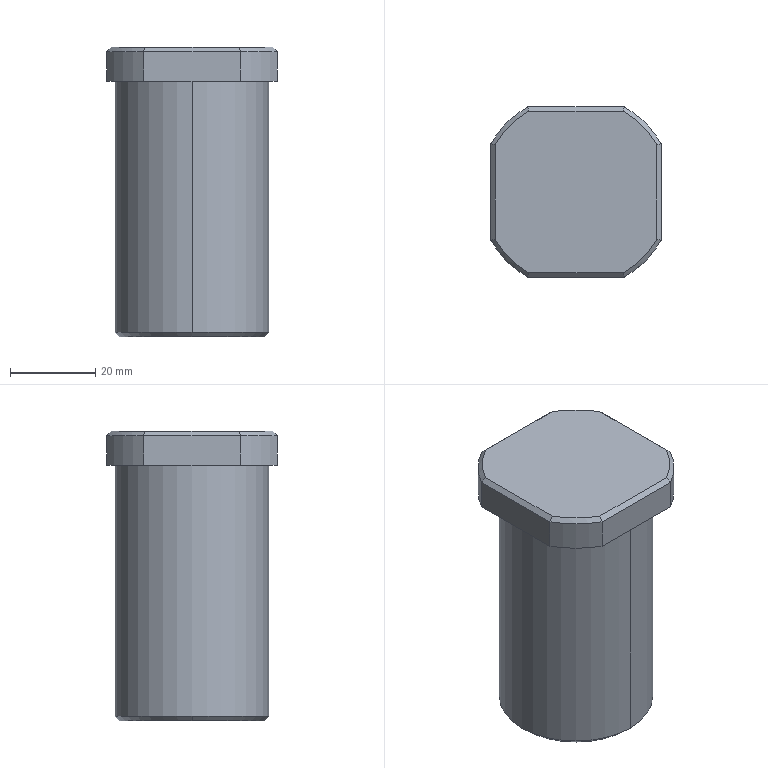Part | Creo | 1 solid | 30 faces | box 40 x 40 x 68 mm | volume 63302 mm3 | plane 12 | cylinder 10 | cone 8 | commonest cylinder face diameters 46 x4 14 x2 16 x2 36 x2
STEP:
#1=CARTESIAN_POINT('',(50.,216.995,-364.));
#2=VERTEX_POINT('',#1);
#3=CARTESIAN_POINT('',(67.,199.995,-364.));
#4=VERTEX_POINT('',#3);
#5=CARTESIAN_POINT('',(50.,199.995,-364.));
#6=DIRECTION('',(0.,0.,-1.));
#7=DIRECTION('',(0.,1.,0.));
#8=AXIS2_PLACEMENT_3D('',#5,#6,#7);
#9=CIRCLE('',#8,17.);
#10=EDGE_CURVE('',#2,#4,#9,.T.);
#11=ORIENTED_EDGE('',*,*,#10,.F.);
#12=CARTESIAN_POINT('',(33.,199.995,-364.));
#13=VERTEX_POINT('',#12);
#14=CARTESIAN_POINT('',(50.,199.995,-364.));
#15=DIRECTION('',(0.,0.,-1.));
#16=DIRECTION('',(-1.,0.,0.));
#17=AXIS2_PLACEMENT_3D('',#14,#15,#16);
#18=CIRCLE('',#17,17.);
#19=EDGE_CURVE('',#13,#2,#18,.T.);
#20=ORIENTED_EDGE('',*,*,#19,.F.);
#21=CARTESIAN_POINT('',(50.,199.995,-364.));
#22=DIRECTION('',(0.,0.,-1.));
#23=DIRECTION('',(1.,0.,0.));
#24=AXIS2_PLACEMENT_3D('',#21,#22,#23);
#25=CIRCLE('',#24,17.);
#26=EDGE_CURVE('',#4,#13,#25,.T.);
#27=ORIENTED_EDGE('',*,*,#26,.F.);
#28=EDGE_LOOP('',(#11,#20,#27));
#29=FACE_OUTER_BOUND('',#28,.F.);
#30=CARTESIAN_POINT('',(42.,199.995,-364.));
#31=VERTEX_POINT('',#30);
#32=CARTESIAN_POINT('',(58.,199.995,-364.));
#33=VERTEX_POINT('',#32);
#34=CARTESIAN_POINT('',(50.,199.995,-364.));
#35=DIRECTION('',(0.,0.,1.));
#36=DIRECTION('',(-1.,0.,0.));
#37=AXIS2_PLACEMENT_3D('',#34,#35,#36);
#38=CIRCLE('',#37,8.);
#39=EDGE_CURVE('',#31,#33,#38,.T.);
#40=ORIENTED_EDGE('',*,*,#39,.F.);
#41=CARTESIAN_POINT('',(50.,199.995,-364.));
#42=DIRECTION('',(0.,0.,1.));
#43=DIRECTION('',(1.,0.,0.));
#44=AXIS2_PLACEMENT_3D('',#41,#42,#43);
#45=CIRCLE('',#44,8.);
#46=EDGE_CURVE('',#33,#31,#45,.T.);
#47=ORIENTED_EDGE('',*,*,#46,.F.);
#48=EDGE_LOOP('',(#40,#47));
#49=FACE_BOUND('',#48,.F.);
#50=CARTESIAN_POINT('',(50.,199.995,-364.));
#51=DIRECTION('',(0.,0.,-1.));
#52=DIRECTION('',(0.,1.,0.));
#53=AXIS2_PLACEMENT_3D('',#50,#51,#52);
#54=PLANE('',#53);
#55=ADVANCED_FACE('',(#29,#49),#54,.T.);
#56=CARTESIAN_POINT('',(50.,217.995,-363.));
#57=VERTEX_POINT('',#56);
#58=CARTESIAN_POINT('',(68.,199.995,-363.));
#59=VERTEX_POINT('',#58);
#60=CARTESIAN_POINT('',(50.,199.995,-363.));
#61=DIRECTION('',(0.,0.,-1.));
#62=DIRECTION('',(0.,1.,0.));
#63=AXIS2_PLACEMENT_3D('',#60,#61,#62);
#64=CIRCLE('',#63,18.);
#65=EDGE_CURVE('',#57,#59,#64,.T.);
#66=ORIENTED_EDGE('',*,*,#65,.F.);
#67=CARTESIAN_POINT('',(32.,199.995,-363.));
#68=VERTEX_POINT('',#67);
#69=CARTESIAN_POINT('',(50.,199.995,-363.));
#70=DIRECTION('',(0.,0.,-1.));
#71=DIRECTION('',(-1.,0.,0.));
#72=AXIS2_PLACEMENT_3D('',#69,#70,#71);
#73=CIRCLE('',#72,18.);
#74=EDGE_CURVE('',#68,#57,#73,.T.);
#75=ORIENTED_EDGE('',*,*,#74,.F.);
#76=CARTESIAN_POINT('',(33.,199.995,-364.));
#77=DIRECTION('',(-0.7071,0.,0.7071));
#78=VECTOR('',#77,1.414);
#79=LINE('',#76,#78);
#80=EDGE_CURVE('',#13,#68,#79,.T.);
#81=ORIENTED_EDGE('',*,*,#80,.F.);
#82=ORIENTED_EDGE('',*,*,#19,.T.);
#83=ORIENTED_EDGE('',*,*,#10,.T.);
#84=CARTESIAN_POINT('',(67.,199.995,-364.));
#85=DIRECTION('',(0.7071,0.,0.7071));
#86=VECTOR('',#85,1.414);
#87=LINE('',#84,#86);
#88=EDGE_CURVE('',#4,#59,#87,.T.);
#89=ORIENTED_EDGE('',*,*,#88,.T.);
#90=EDGE_LOOP('',(#66,#75,#81,#82,#83,#89));
#91=FACE_OUTER_BOUND('',#90,.F.);
#92=CARTESIAN_POINT('',(50.,199.995,-363.5));
#93=DIRECTION('',(0.,0.,1.));
#94=DIRECTION('',(1.,0.,0.));
#95=AXIS2_PLACEMENT_3D('',#92,#93,#94);
#96=CONICAL_SURFACE('',#95,17.5,45.);
#97=ADVANCED_FACE('',(#91),#96,.T.);
#98=CARTESIAN_POINT('',(50.,181.995,-304.));
#99=VERTEX_POINT('',#98);
#100=CARTESIAN_POINT('',(50.,217.995,-304.));
#101=VERTEX_POINT('',#100);
#102=CARTESIAN_POINT('',(50.,199.995,-304.));
#103=DIRECTION('',(0.,0.,1.));
#104=DIRECTION('',(0.,-1.,0.));
#105=AXIS2_PLACEMENT_3D('',#102,#103,#104);
#106=CIRCLE('',#105,18.);
#107=EDGE_CURVE('',#99,#101,#106,.T.);
#108=ORIENTED_EDGE('',*,*,#107,.T.);
#109=CARTESIAN_POINT('',(50.,217.995,-304.));
#110=DIRECTION('',(0.,0.,-1.));
#111=VECTOR('',#110,59.);
#112=LINE('',#109,#111);
#113=EDGE_CURVE('',#101,#57,#112,.T.);
#114=ORIENTED_EDGE('',*,*,#113,.T.);
#115=ORIENTED_EDGE('',*,*,#65,.T.);
#116=CARTESIAN_POINT('',(50.,181.995,-363.));
#117=VERTEX_POINT('',#116);
#118=CARTESIAN_POINT('',(50.,199.995,-363.));
#119=DIRECTION('',(0.,0.,-1.));
#120=DIRECTION('',(1.,0.,0.));
#121=AXIS2_PLACEMENT_3D('',#118,#119,#120);
#122=CIRCLE('',#121,18.);
#123=EDGE_CURVE('',#59,#117,#122,.T.);
#124=ORIENTED_EDGE('',*,*,#123,.T.);
#125=CARTESIAN_POINT('',(50.,181.995,-304.));
#126=DIRECTION('',(0.,0.,-1.));
#127=VECTOR('',#126,59.);
#128=LINE('',#125,#127);
#129=EDGE_CURVE('',#99,#117,#128,.T.);
#130=ORIENTED_EDGE('',*,*,#129,.F.);
#131=EDGE_LOOP('',(#108,#114,#115,#124,#130));
#132=FACE_OUTER_BOUND('',#131,.F.);
#133=CARTESIAN_POINT('',(50.,199.995,-291.1));
#134=DIRECTION('',(0.,0.,-1.));
#135=DIRECTION('',(0.,1.,0.));
#136=AXIS2_PLACEMENT_3D('',#133,#134,#135);
#137=CYLINDRICAL_SURFACE('',#136,18.);
#138=ADVANCED_FACE('',(#132),#137,.T.);
#139=CARTESIAN_POINT('',(70.,188.637,-304.));
#140=VERTEX_POINT('',#139);
#141=CARTESIAN_POINT('',(61.358,179.995,-304.));
#142=VERTEX_POINT('',#141);
#143=CARTESIAN_POINT('',(50.,199.995,-304.));
#144=DIRECTION('',(0.,0.,-1.));
#145=DIRECTION('',(0.8696,-0.4938,0.));
#146=AXIS2_PLACEMENT_3D('',#143,#144,#145);
#147=CIRCLE('',#146,23.);
#148=EDGE_CURVE('',#140,#142,#147,.T.);
#149=ORIENTED_EDGE('',*,*,#148,.F.);
#150=CARTESIAN_POINT('',(70.,211.353,-304.));
#151=VERTEX_POINT('',#150);
#152=CARTESIAN_POINT('',(70.,188.637,-304.));
#153=DIRECTION('',(0.,1.,0.));
#154=VECTOR('',#153,22.716);
#155=LINE('',#152,#154);
#156=EDGE_CURVE('',#140,#151,#155,.T.);
#157=ORIENTED_EDGE('',*,*,#156,.T.);
#158=CARTESIAN_POINT('',(61.358,219.995,-304.));
#159=VERTEX_POINT('',#158);
#160=CARTESIAN_POINT('',(50.,199.995,-304.));
#161=DIRECTION('',(0.,0.,-1.));
#162=DIRECTION('',(0.4938,0.8696,0.));
#163=AXIS2_PLACEMENT_3D('',#160,#161,#162);
#164=CIRCLE('',#163,23.);
#165=EDGE_CURVE('',#159,#151,#164,.T.);
#166=ORIENTED_EDGE('',*,*,#165,.F.);
#167=CARTESIAN_POINT('',(38.642,219.995,-304.));
#168=VERTEX_POINT('',#167);
#169=CARTESIAN_POINT('',(61.358,219.995,-304.));
#170=DIRECTION('',(-1.,0.,0.));
#171=VECTOR('',#170,22.716);
#172=LINE('',#169,#171);
#173=EDGE_CURVE('',#159,#168,#172,.T.);
#174=ORIENTED_EDGE('',*,*,#173,.T.);
#175=CARTESIAN_POINT('',(30.,211.353,-304.));
#176=VERTEX_POINT('',#175);
#177=CARTESIAN_POINT('',(50.,199.995,-304.));
#178=DIRECTION('',(0.,0.,-1.));
#179=DIRECTION('',(-0.8696,0.4938,0.));
#180=AXIS2_PLACEMENT_3D('',#177,#178,#179);
#181=CIRCLE('',#180,23.);
#182=EDGE_CURVE('',#176,#168,#181,.T.);
#183=ORIENTED_EDGE('',*,*,#182,.F.);
#184=CARTESIAN_POINT('',(30.,188.637,-304.));
#185=VERTEX_POINT('',#184);
#186=CARTESIAN_POINT('',(30.,211.353,-304.));
#187=DIRECTION('',(0.,-1.,0.));
#188=VECTOR('',#187,22.716);
#189=LINE('',#186,#188);
#190=EDGE_CURVE('',#176,#185,#189,.T.);
#191=ORIENTED_EDGE('',*,*,#190,.T.);
#192=CARTESIAN_POINT('',(38.642,179.995,-304.));
#193=VERTEX_POINT('',#192);
#194=CARTESIAN_POINT('',(50.,199.995,-304.));
#195=DIRECTION('',(0.,0.,-1.));
#196=DIRECTION('',(-0.4938,-0.8696,0.));
#197=AXIS2_PLACEMENT_3D('',#194,#195,#196);
#198=CIRCLE('',#197,23.);
#199=EDGE_CURVE('',#193,#185,#198,.T.);
#200=ORIENTED_EDGE('',*,*,#199,.F.);
#201=CARTESIAN_POINT('',(38.642,179.995,-304.));
#202=DIRECTION('',(1.,0.,0.));
#203=VECTOR('',#202,22.716);
#204=LINE('',#201,#203);
#205=EDGE_CURVE('',#193,#142,#204,.T.);
#206=ORIENTED_EDGE('',*,*,#205,.T.);
#207=EDGE_LOOP('',(#149,#157,#166,#174,#183,#191,#200,#206));
#208=FACE_OUTER_BOUND('',#207,.F.);
#209=ORIENTED_EDGE('',*,*,#107,.F.);
#210=CARTESIAN_POINT('',(50.,199.995,-304.));
#211=DIRECTION('',(0.,0.,1.));
#212=DIRECTION('',(0.,1.,0.));
#213=AXIS2_PLACEMENT_3D('',#210,#211,#212);
#214=CIRCLE('',#213,18.);
#215=EDGE_CURVE('',#101,#99,#214,.T.);
#216=ORIENTED_EDGE('',*,*,#215,.F.);
#217=EDGE_LOOP('',(#209,#216));
#218=FACE_BOUND('',#217,.F.);
#219=CARTESIAN_POINT('',(50.,199.995,-304.));
#220=DIRECTION('',(0.,0.,-1.));
#221=DIRECTION('',(0.,1.,0.));
#222=AXIS2_PLACEMENT_3D('',#219,#220,#221);
#223=PLANE('',#222);
#224=ADVANCED_FACE('',(#208,#218),#223,.T.);
#225=ORIENTED_EDGE('',*,*,#215,.T.);
#226=ORIENTED_EDGE('',*,*,#129,.T.);
#227=CARTESIAN_POINT('',(50.,199.995,-363.));
#228=DIRECTION('',(0.,0.,-1.));
#229=DIRECTION('',(0.,-1.,0.));
#230=AXIS2_PLACEMENT_3D('',#227,#228,#229);
#231=CIRCLE('',#230,18.);
#232=EDGE_CURVE('',#117,#68,#231,.T.);
#233=ORIENTED_EDGE('',*,*,#232,.T.);
#234=ORIENTED_EDGE('',*,*,#74,.T.);
#235=ORIENTED_EDGE('',*,*,#113,.F.);
#236=EDGE_LOOP('',(#225,#226,#233,#234,#235));
#237=FACE_OUTER_BOUND('',#236,.F.);
#238=CARTESIAN_POINT('',(50.,199.995,-291.1));
#239=DIRECTION('',(0.,0.,-1.));
#240=DIRECTION('',(0.,1.,0.));
#241=AXIS2_PLACEMENT_3D('',#238,#239,#240);
#242=CYLINDRICAL_SURFACE('',#241,18.);
#243=ADVANCED_FACE('',(#237),#242,.T.);
#244=ORIENTED_EDGE('',*,*,#123,.F.);
#245=ORIENTED_EDGE('',*,*,#88,.F.);
#246=ORIENTED_EDGE('',*,*,#26,.T.);
#247=ORIENTED_EDGE('',*,*,#80,.T.);
#248=ORIENTED_EDGE('',*,*,#232,.F.);
#249=EDGE_LOOP('',(#244,#245,#246,#247,#248));
#250=FACE_OUTER_BOUND('',#249,.F.);
#251=CARTESIAN_POINT('',(50.,199.995,-363.5));
#252=DIRECTION('',(0.,0.,1.));
#253=DIRECTION('',(1.,0.,0.));
#254=AXIS2_PLACEMENT_3D('',#251,#252,#253);
#255=CONICAL_SURFACE('',#254,17.5,45.);
#256=ADVANCED_FACE('',(#250),#255,.T.);
#257=CARTESIAN_POINT('',(61.358,179.995,-297.));
#258=VERTEX_POINT('',#257);
#259=CARTESIAN_POINT('',(61.358,179.995,-297.));
#260=DIRECTION('',(-0.000002742,0.000003031,-1.));
#261=VECTOR('',#260,7.);
#262=LINE('',#259,#261);
#263=EDGE_CURVE('',#258,#142,#262,.T.);
#264=ORIENTED_EDGE('',*,*,#263,.F.);
#265=CARTESIAN_POINT('',(70.,188.638,-297.));
#266=VERTEX_POINT('',#265);
#267=CARTESIAN_POINT('',(50.,199.995,-297.));
#268=DIRECTION('',(0.,0.,1.));
#269=DIRECTION('',(0.4938,-0.8696,0.));
#270=AXIS2_PLACEMENT_3D('',#267,#268,#269);
#271=CIRCLE('',#270,22.999);
#272=EDGE_CURVE('',#258,#266,#271,.T.);
#273=ORIENTED_EDGE('',*,*,#272,.T.);
#274=CARTESIAN_POINT('',(70.,188.637,-304.));
#275=DIRECTION('',(0.000003009,0.00001421,1.));
#276=VECTOR('',#275,7.);
#277=LINE('',#274,#276);
#278=EDGE_CURVE('',#140,#266,#277,.T.);
#279=ORIENTED_EDGE('',*,*,#278,.F.);
#280=ORIENTED_EDGE('',*,*,#148,.T.);
#281=EDGE_LOOP('',(#264,#273,#279,#280));
#282=FACE_OUTER_BOUND('',#281,.F.);
#283=CARTESIAN_POINT('',(50.,199.995,-291.1));
#284=DIRECTION('',(0.,0.,-1.));
#285=DIRECTION('',(0.,1.,0.));
#286=AXIS2_PLACEMENT_3D('',#283,#284,#285);
#287=CYLINDRICAL_SURFACE('',#286,23.);
#288=ADVANCED_FACE('',(#282),#287,.T.);
#289=CARTESIAN_POINT('',(38.642,179.995,-297.));
#290=VERTEX_POINT('',#289);
#291=CARTESIAN_POINT('',(38.642,179.995,-304.));
#292=DIRECTION('',(-0.00001537,-0.000001432,1.));
#293=VECTOR('',#292,7.);
#294=LINE('',#291,#293);
#295=EDGE_CURVE('',#193,#290,#294,.T.);
#296=ORIENTED_EDGE('',*,*,#295,.T.);
#297=CARTESIAN_POINT('',(61.358,179.995,-297.));
#298=DIRECTION('',(-1.,0.000000493,0.000000998));
#299=VECTOR('',#298,22.716);
#300=LINE('',#297,#299);
#301=EDGE_CURVE('',#258,#290,#300,.T.);
#302=ORIENTED_EDGE('',*,*,#301,.F.);
#303=ORIENTED_EDGE('',*,*,#263,.T.);
#304=ORIENTED_EDGE('',*,*,#205,.F.);
#305=EDGE_LOOP('',(#296,#302,#303,#304));
#306=FACE_OUTER_BOUND('',#305,.F.);
#307=CARTESIAN_POINT('',(70.,179.995,-296.));
#308=DIRECTION('',(0.,1.,0.));
#309=DIRECTION('',(-1.,0.,0.));
#310=AXIS2_PLACEMENT_3D('',#307,#308,#309);
#311=PLANE('',#310);
#312=ADVANCED_FACE('',(#306),#311,.F.);
#313=CARTESIAN_POINT('',(30.,188.637,-297.));
#314=VERTEX_POINT('',#313);
#315=CARTESIAN_POINT('',(30.,188.637,-297.));
#316=DIRECTION('',(0.000001411,-0.000002038,-1.));
#317=VECTOR('',#316,7.);
#318=LINE('',#315,#317);
#319=EDGE_CURVE('',#314,#185,#318,.T.);
#320=ORIENTED_EDGE('',*,*,#319,.F.);
#321=CARTESIAN_POINT('',(50.001,199.996,-297.));
#322=DIRECTION('',(0.,0.,1.));
#323=DIRECTION('',(-0.8696,-0.4938,0.));
#324=AXIS2_PLACEMENT_3D('',#321,#322,#323);
#325=CIRCLE('',#324,23.001);
#326=EDGE_CURVE('',#314,#290,#325,.T.);
#327=ORIENTED_EDGE('',*,*,#326,.T.);
#328=ORIENTED_EDGE('',*,*,#295,.F.);
#329=ORIENTED_EDGE('',*,*,#199,.T.);
#330=EDGE_LOOP('',(#320,#327,#328,#329));
#331=FACE_OUTER_BOUND('',#330,.F.);
#332=CARTESIAN_POINT('',(50.,199.995,-291.1));
#333=DIRECTION('',(0.,0.,-1.));
#334=DIRECTION('',(0.,1.,0.));
#335=AXIS2_PLACEMENT_3D('',#332,#333,#334);
#336=CYLINDRICAL_SURFACE('',#335,23.);
#337=ADVANCED_FACE('',(#331),#336,.T.);
#338=CARTESIAN_POINT('',(30.,211.353,-297.));
#339=VERTEX_POINT('',#338);
#340=CARTESIAN_POINT('',(30.,211.353,-304.));
#341=DIRECTION('',(-0.000003011,-0.00001424,1.));
#342=VECTOR('',#341,7.);
#343=LINE('',#340,#342);
#344=EDGE_CURVE('',#176,#339,#343,.T.);
#345=ORIENTED_EDGE('',*,*,#344,.T.);
#346=CARTESIAN_POINT('',(30.,188.637,-297.));
#347=DIRECTION('',(-0.000000493,1.,-0.000000999));
#348=VECTOR('',#347,22.716);
#349=LINE('',#346,#348);
#350=EDGE_CURVE('',#314,#339,#349,.T.);
#351=ORIENTED_EDGE('',*,*,#350,.F.);
#352=ORIENTED_EDGE('',*,*,#319,.T.);
#353=ORIENTED_EDGE('',*,*,#190,.F.);
#354=EDGE_LOOP('',(#345,#351,#352,#353));
#355=FACE_OUTER_BOUND('',#354,.F.);
#356=CARTESIAN_POINT('',(30.,179.995,-296.));
#357=DIRECTION('',(1.,0.,0.));
#358=DIRECTION('',(0.,1.,0.));
#359=AXIS2_PLACEMENT_3D('',#356,#357,#358);
#360=PLANE('',#359);
#361=ADVANCED_FACE('',(#355),#360,.F.);
#362=CARTESIAN_POINT('',(38.642,219.995,-297.));
#363=VERTEX_POINT('',#362);
#364=CARTESIAN_POINT('',(38.642,219.995,-297.));
#365=DIRECTION('',(0.000002746,-0.000003033,-1.));
#366=VECTOR('',#365,7.);
#367=LINE('',#364,#366);
#368=EDGE_CURVE('',#363,#168,#367,.T.);
#369=ORIENTED_EDGE('',*,*,#368,.F.);
#370=CARTESIAN_POINT('',(50.,199.996,-297.));
#371=DIRECTION('',(0.,0.,1.));
#372=DIRECTION('',(-0.4938,0.8696,0.));
#373=AXIS2_PLACEMENT_3D('',#370,#371,#372);
#374=CIRCLE('',#373,22.999);
#375=EDGE_CURVE('',#363,#339,#374,.T.);
#376=ORIENTED_EDGE('',*,*,#375,.T.);
#377=ORIENTED_EDGE('',*,*,#344,.F.);
#378=ORIENTED_EDGE('',*,*,#182,.T.);
#379=EDGE_LOOP('',(#369,#376,#377,#378));
#380=FACE_OUTER_BOUND('',#379,.F.);
#381=CARTESIAN_POINT('',(50.,199.995,-291.1));
#382=DIRECTION('',(0.,0.,-1.));
#383=DIRECTION('',(0.,1.,0.));
#384=AXIS2_PLACEMENT_3D('',#381,#382,#383);
#385=CYLINDRICAL_SURFACE('',#384,23.);
#386=ADVANCED_FACE('',(#380),#385,.T.);
#387=CARTESIAN_POINT('',(61.358,219.995,-297.));
#388=VERTEX_POINT('',#387);
#389=CARTESIAN_POINT('',(61.358,219.995,-304.));
#390=DIRECTION('',(0.0000153,0.000001435,1.));
#391=VECTOR('',#390,7.);
#392=LINE('',#389,#391);
#393=EDGE_CURVE('',#159,#388,#392,.T.);
#394=ORIENTED_EDGE('',*,*,#393,.T.);
#395=CARTESIAN_POINT('',(38.642,219.995,-297.));
#396=DIRECTION('',(1.,-0.000000492,0.000000996));
#397=VECTOR('',#396,22.716);
#398=LINE('',#395,#397);
#399=EDGE_CURVE('',#363,#388,#398,.T.);
#400=ORIENTED_EDGE('',*,*,#399,.F.);
#401=ORIENTED_EDGE('',*,*,#368,.T.);
#402=ORIENTED_EDGE('',*,*,#173,.F.);
#403=EDGE_LOOP('',(#394,#400,#401,#402));
#404=FACE_OUTER_BOUND('',#403,.F.);
#405=CARTESIAN_POINT('',(30.,219.995,-296.));
#406=DIRECTION('',(0.,-1.,0.));
#407=DIRECTION('',(1.,0.,0.));
#408=AXIS2_PLACEMENT_3D('',#405,#406,#407);
#409=PLANE('',#408);
#410=ADVANCED_FACE('',(#404),#409,.F.);
#411=CARTESIAN_POINT('',(70.,211.353,-297.));
#412=VERTEX_POINT('',#411);
#413=CARTESIAN_POINT('',(70.,211.353,-297.));
#414=DIRECTION('',(-0.000001415,0.000002027,-1.));
#415=VECTOR('',#414,7.);
#416=LINE('',#413,#415);
#417=EDGE_CURVE('',#412,#151,#416,.T.);
#418=ORIENTED_EDGE('',*,*,#417,.F.);
#419=CARTESIAN_POINT('',(49.999,199.995,-297.));
#420=DIRECTION('',(0.,0.,1.));
#421=DIRECTION('',(0.8696,0.4938,0.));
#422=AXIS2_PLACEMENT_3D('',#419,#420,#421);
#423=CIRCLE('',#422,23.001);
#424=EDGE_CURVE('',#412,#388,#423,.T.);
#425=ORIENTED_EDGE('',*,*,#424,.T.);
#426=ORIENTED_EDGE('',*,*,#393,.F.);
#427=ORIENTED_EDGE('',*,*,#165,.T.);
#428=EDGE_LOOP('',(#418,#425,#426,#427));
#429=FACE_OUTER_BOUND('',#428,.F.);
#430=CARTESIAN_POINT('',(50.,199.995,-291.1));
#431=DIRECTION('',(0.,0.,-1.));
#432=DIRECTION('',(0.,1.,0.));
#433=AXIS2_PLACEMENT_3D('',#430,#431,#432);
#434=CYLINDRICAL_SURFACE('',#433,23.);
#435=ADVANCED_FACE('',(#429),#434,.T.);
#436=ORIENTED_EDGE('',*,*,#278,.T.);
#437=CARTESIAN_POINT('',(70.,211.353,-297.));
#438=DIRECTION('',(0.000000491,-1.,-0.000000995));
#439=VECTOR('',#438,22.716);
#440=LINE('',#437,#439);
#441=EDGE_CURVE('',#412,#266,#440,.T.);
#442=ORIENTED_EDGE('',*,*,#441,.F.);
#443=ORIENTED_EDGE('',*,*,#417,.T.);
#444=ORIENTED_EDGE('',*,*,#156,.F.);
#445=EDGE_LOOP('',(#436,#442,#443,#444));
#446=FACE_OUTER_BOUND('',#445,.F.);
#447=CARTESIAN_POINT('',(70.,219.995,-296.));
#448=DIRECTION('',(-1.,0.,0.));
#449=DIRECTION('',(0.,-1.,0.));
#450=AXIS2_PLACEMENT_3D('',#447,#448,#449);
#451=PLANE('',#450);
#452=ADVANCED_FACE('',(#446),#451,.F.);
#453=CARTESIAN_POINT('',(69.,211.086,-296.));
#454=VERTEX_POINT('',#453);
#455=CARTESIAN_POINT('',(69.11,211.116,-296.11));
#456=CARTESIAN_POINT('',(69.331,211.175,-296.331));
#457=CARTESIAN_POINT('',(69.664,211.264,-296.665));
#458=CARTESIAN_POINT('',(69.888,211.324,-296.888));
#459=CARTESIAN_POINT('',(70.,211.353,-297.));
#460=B_SPLINE_CURVE_WITH_KNOTS('',3,(#453,#455,#456,#457,#458,#459),.UNSPECIFIED.,.F.,.F.,(4,1,1,4),(0.,0.3333,0.6667,1.),.UNSPECIFIED.);
#461=EDGE_CURVE('',#454,#412,#460,.T.);
#462=ORIENTED_EDGE('',*,*,#461,.T.);
#463=ORIENTED_EDGE('',*,*,#441,.T.);
#464=CARTESIAN_POINT('',(69.,188.905,-296.));
#465=VERTEX_POINT('',#464);
#466=CARTESIAN_POINT('',(69.,188.905,-296.));
#467=CARTESIAN_POINT('',(69.11,188.875,-296.11));
#468=CARTESIAN_POINT('',(69.332,188.815,-296.332));
#469=CARTESIAN_POINT('',(69.665,188.726,-296.665));
#470=CARTESIAN_POINT('',(69.888,188.667,-296.888));
#471=CARTESIAN_POINT('',(70.,188.638,-297.));
#472=B_SPLINE_CURVE_WITH_KNOTS('',3,(#466,#467,#468,#469,#470,#471),.UNSPECIFIED.,.F.,.F.,(4,1,1,4),(0.,0.3333,0.6667,1.),.UNSPECIFIED.);
#473=EDGE_CURVE('',#465,#266,#472,.T.);
#474=ORIENTED_EDGE('',*,*,#473,.F.);
#475=CARTESIAN_POINT('',(69.,211.086,-296.));
#476=DIRECTION('',(0.000000013,-1.,0.));
#477=VECTOR('',#476,22.181);
#478=LINE('',#475,#477);
#479=EDGE_CURVE('',#454,#465,#478,.T.);
#480=ORIENTED_EDGE('',*,*,#479,.F.);
#481=EDGE_LOOP('',(#462,#463,#474,#480));
#482=FACE_OUTER_BOUND('',#481,.F.);
#483=CARTESIAN_POINT('',(69.5,199.995,-296.5));
#484=DIRECTION('',(0.7071,0.,0.7071));
#485=DIRECTION('',(0.7071,0.,-0.7071));
#486=AXIS2_PLACEMENT_3D('',#483,#484,#485);
#487=PLANE('',#486);
#488=ADVANCED_FACE('',(#482),#487,.T.);
#489=ORIENTED_EDGE('',*,*,#461,.F.);
#490=CARTESIAN_POINT('',(61.091,218.995,-296.));
#491=VERTEX_POINT('',#490);
#492=CARTESIAN_POINT('',(49.999,199.995,-296.));
#493=DIRECTION('',(0.,0.,1.));
#494=DIRECTION('',(0.8636,0.5041,0.));
#495=AXIS2_PLACEMENT_3D('',#492,#493,#494);
#496=CIRCLE('',#495,22.001);
#497=EDGE_CURVE('',#454,#491,#496,.T.);
#498=ORIENTED_EDGE('',*,*,#497,.T.);
#499=CARTESIAN_POINT('',(61.121,219.105,-296.11));
#500=CARTESIAN_POINT('',(61.18,219.326,-296.331));
#501=CARTESIAN_POINT('',(61.269,219.659,-296.664));
#502=CARTESIAN_POINT('',(61.328,219.883,-296.888));
#503=CARTESIAN_POINT('',(61.358,219.995,-297.));
#504=B_SPLINE_CURVE_WITH_KNOTS('',3,(#490,#499,#500,#501,#502,#503),.UNSPECIFIED.,.F.,.F.,(4,1,1,4),(0.,0.3333,0.6667,1.),.UNSPECIFIED.);
#505=EDGE_CURVE('',#491,#388,#504,.T.);
#506=ORIENTED_EDGE('',*,*,#505,.T.);
#507=ORIENTED_EDGE('',*,*,#424,.F.);
#508=EDGE_LOOP('',(#489,#498,#506,#507));
#509=FACE_OUTER_BOUND('',#508,.F.);
#510=CARTESIAN_POINT('',(49.999,199.995,-296.5));
#511=DIRECTION('',(0.,0.,-1.));
#512=DIRECTION('',(1.,0.,0.));
#513=AXIS2_PLACEMENT_3D('',#510,#511,#512);
#514=CONICAL_SURFACE('',#513,22.501,45.);
#515=ADVANCED_FACE('',(#509),#514,.T.);
#516=CARTESIAN_POINT('',(38.909,218.995,-296.));
#517=VERTEX_POINT('',#516);
#518=CARTESIAN_POINT('',(38.909,218.995,-296.));
#519=DIRECTION('',(1.,0.,0.));
#520=VECTOR('',#519,22.181);
#521=LINE('',#518,#520);
#522=EDGE_CURVE('',#517,#491,#521,.T.);
#523=ORIENTED_EDGE('',*,*,#522,.T.);
#524=ORIENTED_EDGE('',*,*,#497,.F.);
#525=ORIENTED_EDGE('',*,*,#479,.T.);
#526=CARTESIAN_POINT('',(61.091,180.995,-296.));
#527=VERTEX_POINT('',#526);
#528=CARTESIAN_POINT('',(50.,199.995,-296.));
#529=DIRECTION('',(0.,0.,1.));
#530=DIRECTION('',(0.5041,-0.8636,0.));
#531=AXIS2_PLACEMENT_3D('',#528,#529,#530);
#532=CIRCLE('',#531,21.999);
#533=EDGE_CURVE('',#527,#465,#532,.T.);
#534=ORIENTED_EDGE('',*,*,#533,.F.);
#535=CARTESIAN_POINT('',(38.909,180.995,-296.));
#536=VERTEX_POINT('',#535);
#537=CARTESIAN_POINT('',(61.091,180.995,-296.));
#538=DIRECTION('',(-1.,0.,0.));
#539=VECTOR('',#538,22.181);
#540=LINE('',#537,#539);
#541=EDGE_CURVE('',#527,#536,#540,.T.);
#542=ORIENTED_EDGE('',*,*,#541,.T.);
#543=CARTESIAN_POINT('',(31.,188.905,-296.));
#544=VERTEX_POINT('',#543);
#545=CARTESIAN_POINT('',(50.001,199.996,-296.));
#546=DIRECTION('',(0.,0.,1.));
#547=DIRECTION('',(-0.8636,-0.5041,0.));
#548=AXIS2_PLACEMENT_3D('',#545,#546,#547);
#549=CIRCLE('',#548,22.001);
#550=EDGE_CURVE('',#544,#536,#549,.T.);
#551=ORIENTED_EDGE('',*,*,#550,.F.);
#552=CARTESIAN_POINT('',(31.,211.086,-296.));
#553=VERTEX_POINT('',#552);
#554=CARTESIAN_POINT('',(31.,188.905,-296.));
#555=DIRECTION('',(-0.000000013,1.,0.));
#556=VECTOR('',#555,22.181);
#557=LINE('',#554,#556);
#558=EDGE_CURVE('',#544,#553,#557,.T.);
#559=ORIENTED_EDGE('',*,*,#558,.T.);
#560=CARTESIAN_POINT('',(50.,199.996,-296.));
#561=DIRECTION('',(0.,0.,1.));
#562=DIRECTION('',(-0.5041,0.8636,0.));
#563=AXIS2_PLACEMENT_3D('',#560,#561,#562);
#564=CIRCLE('',#563,21.999);
#565=EDGE_CURVE('',#517,#553,#564,.T.);
#566=ORIENTED_EDGE('',*,*,#565,.F.);
#567=EDGE_LOOP('',(#523,#524,#525,#534,#542,#551,#559,#566));
#568=FACE_OUTER_BOUND('',#567,.F.);
#569=CARTESIAN_POINT('',(50.,199.995,-296.));
#570=DIRECTION('',(0.,0.,-1.));
#571=DIRECTION('',(0.,1.,0.));
#572=AXIS2_PLACEMENT_3D('',#569,#570,#571);
#573=PLANE('',#572);
#574=ADVANCED_FACE('',(#568),#573,.F.);
#575=ORIENTED_EDGE('',*,*,#505,.F.);
#576=ORIENTED_EDGE('',*,*,#522,.F.);
#577=CARTESIAN_POINT('',(38.88,219.105,-296.11));
#578=CARTESIAN_POINT('',(38.82,219.326,-296.331));
#579=CARTESIAN_POINT('',(38.731,219.66,-296.664));
#580=CARTESIAN_POINT('',(38.672,219.883,-296.888));
#581=CARTESIAN_POINT('',(38.642,219.995,-297.));
#582=B_SPLINE_CURVE_WITH_KNOTS('',3,(#516,#577,#578,#579,#580,#581),.UNSPECIFIED.,.F.,.F.,(4,1,1,4),(0.,0.3333,0.6667,1.),.UNSPECIFIED.);
#583=EDGE_CURVE('',#517,#363,#582,.T.);
#584=ORIENTED_EDGE('',*,*,#583,.T.);
#585=ORIENTED_EDGE('',*,*,#399,.T.);
#586=EDGE_LOOP('',(#575,#576,#584,#585));
#587=FACE_OUTER_BOUND('',#586,.F.);
#588=CARTESIAN_POINT('',(50.,219.495,-296.5));
#589=DIRECTION('',(0.,0.7071,0.7071));
#590=DIRECTION('',(0.,0.7071,-0.7071));
#591=AXIS2_PLACEMENT_3D('',#588,#589,#590);
#592=PLANE('',#591);
#593=ADVANCED_FACE('',(#587),#592,.T.);
#594=ORIENTED_EDGE('',*,*,#583,.F.);
#595=ORIENTED_EDGE('',*,*,#565,.T.);
#596=CARTESIAN_POINT('',(30.,211.353,-297.));
#597=CARTESIAN_POINT('',(30.112,211.323,-296.888));
#598=CARTESIAN_POINT('',(30.335,211.264,-296.665));
#599=CARTESIAN_POINT('',(30.668,211.175,-296.332));
#600=CARTESIAN_POINT('',(30.89,211.116,-296.11));
#601=B_SPLINE_CURVE_WITH_KNOTS('',3,(#596,#597,#598,#599,#600,#552),.UNSPECIFIED.,.F.,.F.,(4,1,1,4),(0.,0.3333,0.6667,1.),.UNSPECIFIED.);
#602=EDGE_CURVE('',#339,#553,#601,.T.);
#603=ORIENTED_EDGE('',*,*,#602,.F.);
#604=ORIENTED_EDGE('',*,*,#375,.F.);
#605=EDGE_LOOP('',(#594,#595,#603,#604));
#606=FACE_OUTER_BOUND('',#605,.F.);
#607=CARTESIAN_POINT('',(50.,199.996,-296.5));
#608=DIRECTION('',(0.,0.,-1.));
#609=DIRECTION('',(1.,0.,0.));
#610=AXIS2_PLACEMENT_3D('',#607,#608,#609);
#611=CONICAL_SURFACE('',#610,22.499,45.);
#612=ADVANCED_FACE('',(#606),#611,.T.);
#613=ORIENTED_EDGE('',*,*,#602,.T.);
#614=ORIENTED_EDGE('',*,*,#558,.F.);
#615=CARTESIAN_POINT('',(30.89,188.875,-296.11));
#616=CARTESIAN_POINT('',(30.669,188.815,-296.331));
#617=CARTESIAN_POINT('',(30.336,188.726,-296.665));
#618=CARTESIAN_POINT('',(30.112,188.667,-296.888));
#619=CARTESIAN_POINT('',(30.,188.637,-297.));
#620=B_SPLINE_CURVE_WITH_KNOTS('',3,(#543,#615,#616,#617,#618,#619),.UNSPECIFIED.,.F.,.F.,(4,1,1,4),(0.,0.3333,0.6667,1.),.UNSPECIFIED.);
#621=EDGE_CURVE('',#544,#314,#620,.T.);
#622=ORIENTED_EDGE('',*,*,#621,.T.);
#623=ORIENTED_EDGE('',*,*,#350,.T.);
#624=EDGE_LOOP('',(#613,#614,#622,#623));
#625=FACE_OUTER_BOUND('',#624,.F.);
#626=CARTESIAN_POINT('',(30.5,199.995,-296.5));
#627=DIRECTION('',(-0.7071,0.,0.7071));
#628=DIRECTION('',(-0.7071,0.,-0.7071));
#629=AXIS2_PLACEMENT_3D('',#626,#627,#628);
#630=PLANE('',#629);
#631=ADVANCED_FACE('',(#625),#630,.T.);
#632=ORIENTED_EDGE('',*,*,#621,.F.);
#633=ORIENTED_EDGE('',*,*,#550,.T.);
#634=CARTESIAN_POINT('',(38.642,179.995,-297.));
#635=CARTESIAN_POINT('',(38.672,180.107,-296.888));
#636=CARTESIAN_POINT('',(38.731,180.331,-296.664));
#637=CARTESIAN_POINT('',(38.82,180.664,-296.331));
#638=CARTESIAN_POINT('',(38.879,180.885,-296.11));
#639=CARTESIAN_POINT('',(38.909,180.995,-296.));
#640=B_SPLINE_CURVE_WITH_KNOTS('',3,(#634,#635,#636,#637,#638,#639),.UNSPECIFIED.,.F.,.F.,(4,1,1,4),(0.,0.3333,0.6667,1.),.UNSPECIFIED.);
#641=EDGE_CURVE('',#290,#536,#640,.T.);
#642=ORIENTED_EDGE('',*,*,#641,.F.);
#643=ORIENTED_EDGE('',*,*,#326,.F.);
#644=EDGE_LOOP('',(#632,#633,#642,#643));
#645=FACE_OUTER_BOUND('',#644,.F.);
#646=CARTESIAN_POINT('',(50.001,199.996,-296.5));
#647=DIRECTION('',(0.,0.,-1.));
#648=DIRECTION('',(1.,0.,0.));
#649=AXIS2_PLACEMENT_3D('',#646,#647,#648);
#650=CONICAL_SURFACE('',#649,22.501,45.);
#651=ADVANCED_FACE('',(#645),#650,.T.);
#652=CARTESIAN_POINT('',(61.12,180.885,-296.11));
#653=CARTESIAN_POINT('',(61.18,180.664,-296.331));
#654=CARTESIAN_POINT('',(61.269,180.331,-296.664));
#655=CARTESIAN_POINT('',(61.328,180.107,-296.888));
#656=CARTESIAN_POINT('',(61.358,179.995,-297.));
#657=B_SPLINE_CURVE_WITH_KNOTS('',3,(#526,#652,#653,#654,#655,#656),.UNSPECIFIED.,.F.,.F.,(4,1,1,4),(0.,0.3333,0.6667,1.),.UNSPECIFIED.);
#658=EDGE_CURVE('',#527,#258,#657,.T.);
#659=ORIENTED_EDGE('',*,*,#658,.T.);
#660=ORIENTED_EDGE('',*,*,#301,.T.);
#661=ORIENTED_EDGE('',*,*,#641,.T.);
#662=ORIENTED_EDGE('',*,*,#541,.F.);
#663=EDGE_LOOP('',(#659,#660,#661,#662));
#664=FACE_OUTER_BOUND('',#663,.F.);
#665=CARTESIAN_POINT('',(50.,180.495,-296.5));
#666=DIRECTION('',(0.,-0.7071,0.7071));
#667=DIRECTION('',(0.,-0.7071,-0.7071));
#668=AXIS2_PLACEMENT_3D('',#665,#666,#667);
#669=PLANE('',#668);
#670=ADVANCED_FACE('',(#664),#669,.T.);
#671=ORIENTED_EDGE('',*,*,#658,.F.);
#672=ORIENTED_EDGE('',*,*,#533,.T.);
#673=ORIENTED_EDGE('',*,*,#473,.T.);
#674=ORIENTED_EDGE('',*,*,#272,.F.);
#675=EDGE_LOOP('',(#671,#672,#673,#674));
#676=FACE_OUTER_BOUND('',#675,.F.);
#677=CARTESIAN_POINT('',(50.,199.995,-296.5));
#678=DIRECTION('',(0.,0.,-1.));
#679=DIRECTION('',(1.,0.,0.));
#680=AXIS2_PLACEMENT_3D('',#677,#678,#679);
#681=CONICAL_SURFACE('',#680,22.499,45.);
#682=ADVANCED_FACE('',(#676),#681,.T.);
#683=CARTESIAN_POINT('',(58.,199.995,-321.));
#684=VERTEX_POINT('',#683);
#685=CARTESIAN_POINT('',(42.,199.995,-321.));
#686=VERTEX_POINT('',#685);
#687=CARTESIAN_POINT('',(50.,199.995,-321.));
#688=DIRECTION('',(0.,0.,-1.));
#689=DIRECTION('',(1.,0.,0.));
#690=AXIS2_PLACEMENT_3D('',#687,#688,#689);
#691=CIRCLE('',#690,8.);
#692=EDGE_CURVE('',#684,#686,#691,.T.);
#693=ORIENTED_EDGE('',*,*,#692,.T.);
#694=CARTESIAN_POINT('',(42.,199.995,-364.));
#695=DIRECTION('',(0.,0.,1.));
#696=VECTOR('',#695,43.);
#697=LINE('',#694,#696);
#698=EDGE_CURVE('',#31,#686,#697,.T.);
#699=ORIENTED_EDGE('',*,*,#698,.F.);
#700=ORIENTED_EDGE('',*,*,#39,.T.);
#701=CARTESIAN_POINT('',(58.,199.995,-364.));
#702=DIRECTION('',(0.,0.,1.));
#703=VECTOR('',#702,43.);
#704=LINE('',#701,#703);
#705=EDGE_CURVE('',#33,#684,#704,.T.);
#706=ORIENTED_EDGE('',*,*,#705,.T.);
#707=EDGE_LOOP('',(#693,#699,#700,#706));
#708=FACE_OUTER_BOUND('',#707,.F.);
#709=CARTESIAN_POINT('',(50.,199.995,-366.));
#710=DIRECTION('',(0.,0.,1.));
#711=DIRECTION('',(-1.,0.,0.));
#712=AXIS2_PLACEMENT_3D('',#709,#710,#711);
#713=CYLINDRICAL_SURFACE('',#712,8.);
#714=ADVANCED_FACE('',(#708),#713,.F.);
#715=ORIENTED_EDGE('',*,*,#692,.F.);
#716=CARTESIAN_POINT('',(50.,199.995,-321.));
#717=DIRECTION('',(0.,0.,-1.));
#718=DIRECTION('',(-1.,0.,0.));
#719=AXIS2_PLACEMENT_3D('',#716,#717,#718);
#720=CIRCLE('',#719,8.);
#721=EDGE_CURVE('',#686,#684,#720,.T.);
#722=ORIENTED_EDGE('',*,*,#721,.F.);
#723=EDGE_LOOP('',(#715,#722));
#724=FACE_OUTER_BOUND('',#723,.F.);
#725=CARTESIAN_POINT('',(57.,199.995,-321.));
#726=VERTEX_POINT('',#725);
#727=CARTESIAN_POINT('',(43.,199.995,-321.));
#728=VERTEX_POINT('',#727);
#729=CARTESIAN_POINT('',(50.,199.995,-321.));
#730=DIRECTION('',(0.,0.,1.));
#731=DIRECTION('',(1.,0.,0.));
#732=AXIS2_PLACEMENT_3D('',#729,#730,#731);
#733=CIRCLE('',#732,7.);
#734=EDGE_CURVE('',#726,#728,#733,.T.);
#735=ORIENTED_EDGE('',*,*,#734,.F.);
#736=CARTESIAN_POINT('',(50.,199.995,-321.));
#737=DIRECTION('',(0.,0.,1.));
#738=DIRECTION('',(-1.,0.,0.));
#739=AXIS2_PLACEMENT_3D('',#736,#737,#738);
#740=CIRCLE('',#739,7.);
#741=EDGE_CURVE('',#728,#726,#740,.T.);
#742=ORIENTED_EDGE('',*,*,#741,.F.);
#743=EDGE_LOOP('',(#735,#742));
#744=FACE_BOUND('',#743,.F.);
#745=CARTESIAN_POINT('',(50.,199.995,-321.));
#746=DIRECTION('',(0.,0.,1.));
#747=DIRECTION('',(-1.,0.,0.));
#748=AXIS2_PLACEMENT_3D('',#745,#746,#747);
#749=PLANE('',#748);
#750=ADVANCED_FACE('',(#724,#744),#749,.F.);
#751=CARTESIAN_POINT('',(43.,199.995,-318.));
#752=VERTEX_POINT('',#751);
#753=CARTESIAN_POINT('',(57.,199.995,-318.));
#754=VERTEX_POINT('',#753);
#755=CARTESIAN_POINT('',(50.,199.995,-318.));
#756=DIRECTION('',(0.,0.,-1.));
#757=DIRECTION('',(-1.,0.,0.));
#758=AXIS2_PLACEMENT_3D('',#755,#756,#757);
#759=CIRCLE('',#758,7.);
#760=EDGE_CURVE('',#752,#754,#759,.T.);
#761=ORIENTED_EDGE('',*,*,#760,.T.);
#762=CARTESIAN_POINT('',(57.,199.995,-321.));
#763=DIRECTION('',(0.,0.,1.));
#764=VECTOR('',#763,3.);
#765=LINE('',#762,#764);
#766=EDGE_CURVE('',#726,#754,#765,.T.);
#767=ORIENTED_EDGE('',*,*,#766,.F.);
#768=ORIENTED_EDGE('',*,*,#734,.T.);
#769=CARTESIAN_POINT('',(43.,199.995,-321.));
#770=DIRECTION('',(0.,0.,1.));
#771=VECTOR('',#770,3.);
#772=LINE('',#769,#771);
#773=EDGE_CURVE('',#728,#752,#772,.T.);
#774=ORIENTED_EDGE('',*,*,#773,.T.);
#775=EDGE_LOOP('',(#761,#767,#768,#774));
#776=FACE_OUTER_BOUND('',#775,.F.);
#777=CARTESIAN_POINT('',(50.,199.995,-321.));
#778=DIRECTION('',(0.,0.,1.));
#779=DIRECTION('',(-1.,0.,0.));
#780=AXIS2_PLACEMENT_3D('',#777,#778,#779);
#781=CYLINDRICAL_SURFACE('',#780,7.);
#782=ADVANCED_FACE('',(#776),#781,.F.);
#783=ORIENTED_EDGE('',*,*,#760,.F.);
#784=CARTESIAN_POINT('',(50.,199.995,-311.));
#785=VERTEX_POINT('',#784);
#786=CARTESIAN_POINT('',(50.,199.995,-311.));
#787=DIRECTION('',(-0.7071,0.,-0.7071));
#788=VECTOR('',#787,9.899);
#789=LINE('',#786,#788);
#790=EDGE_CURVE('',#785,#752,#789,.T.);
#791=ORIENTED_EDGE('',*,*,#790,.F.);
#792=CARTESIAN_POINT('',(50.,199.995,-311.));
#793=DIRECTION('',(0.7071,0.,-0.7071));
#794=VECTOR('',#793,9.899);
#795=LINE('',#792,#794);
#796=EDGE_CURVE('',#785,#754,#795,.T.);
#797=ORIENTED_EDGE('',*,*,#796,.T.);
#798=EDGE_LOOP('',(#783,#791,#797));
#799=FACE_OUTER_BOUND('',#798,.F.);
#800=CARTESIAN_POINT('',(50.,199.995,-314.57));
#801=DIRECTION('',(0.,0.,-1.));
#802=DIRECTION('',(1.,0.,0.));
#803=AXIS2_PLACEMENT_3D('',#800,#801,#802);
#804=CONICAL_SURFACE('',#803,3.57,45.);
#805=ADVANCED_FACE('',(#799),#804,.F.);
#806=CARTESIAN_POINT('',(50.,199.995,-318.));
#807=DIRECTION('',(0.,0.,-1.));
#808=DIRECTION('',(1.,0.,0.));
#809=AXIS2_PLACEMENT_3D('',#806,#807,#808);
#810=CIRCLE('',#809,7.);
#811=EDGE_CURVE('',#754,#752,#810,.T.);
#812=ORIENTED_EDGE('',*,*,#811,.F.);
#813=ORIENTED_EDGE('',*,*,#796,.F.);
#814=ORIENTED_EDGE('',*,*,#790,.T.);
#815=EDGE_LOOP('',(#812,#813,#814));
#816=FACE_OUTER_BOUND('',#815,.F.);
#817=CARTESIAN_POINT('',(50.,199.995,-314.57));
#818=DIRECTION('',(0.,0.,-1.));
#819=DIRECTION('',(1.,0.,0.));
#820=AXIS2_PLACEMENT_3D('',#817,#818,#819);
#821=CONICAL_SURFACE('',#820,3.57,45.);
#822=ADVANCED_FACE('',(#816),#821,.F.);
#823=ORIENTED_EDGE('',*,*,#811,.T.);
#824=ORIENTED_EDGE('',*,*,#773,.F.);
#825=ORIENTED_EDGE('',*,*,#741,.T.);
#826=ORIENTED_EDGE('',*,*,#766,.T.);
#827=EDGE_LOOP('',(#823,#824,#825,#826));
#828=FACE_OUTER_BOUND('',#827,.F.);
#829=CARTESIAN_POINT('',(50.,199.995,-321.));
#830=DIRECTION('',(0.,0.,1.));
#831=DIRECTION('',(-1.,0.,0.));
#832=AXIS2_PLACEMENT_3D('',#829,#830,#831);
#833=CYLINDRICAL_SURFACE('',#832,7.);
#834=ADVANCED_FACE('',(#828),#833,.F.);
#835=ORIENTED_EDGE('',*,*,#721,.T.);
#836=ORIENTED_EDGE('',*,*,#705,.F.);
#837=ORIENTED_EDGE('',*,*,#46,.T.);
#838=ORIENTED_EDGE('',*,*,#698,.T.);
#839=EDGE_LOOP('',(#835,#836,#837,#838));
#840=FACE_OUTER_BOUND('',#839,.F.);
#841=CARTESIAN_POINT('',(50.,199.995,-366.));
#842=DIRECTION('',(0.,0.,1.));
#843=DIRECTION('',(-1.,0.,0.));
#844=AXIS2_PLACEMENT_3D('',#841,#842,#843);
#845=CYLINDRICAL_SURFACE('',#844,8.);
#846=ADVANCED_FACE('',(#840),#845,.F.);
#847=CLOSED_SHELL('',(#55,#97,#138,#224,#243,#256,#288,#312,#337,#361,#386,#410,#435,#452,#488,#515,#574,#593,#612,#631,#651,#670,#682,#714,#750,#782,#805,#822,#834,#846));
#848=MANIFOLD_SOLID_BREP('',#847);
#849=(LENGTH_UNIT()NAMED_UNIT(*)SI_UNIT(.MILLI.,.METRE.));
#850=UNCERTAINTY_MEASURE_WITH_UNIT(LENGTH_MEASURE(0.008845),#849,'','');
#851=(NAMED_UNIT(*)PLANE_ANGLE_UNIT()SI_UNIT($,.RADIAN.));
#852=PLANE_ANGLE_MEASURE_WITH_UNIT(PLANE_ANGLE_MEASURE(0.01745),#851);
#853=(CONVERSION_BASED_UNIT('DEGREE',#852)NAMED_UNIT(*)PLANE_ANGLE_UNIT());
#854=(NAMED_UNIT(*)SI_UNIT($,.STERADIAN.)SOLID_ANGLE_UNIT());
#855=(GEOMETRIC_REPRESENTATION_CONTEXT(3)GLOBAL_UNCERTAINTY_ASSIGNED_CONTEXT((#850))GLOBAL_UNIT_ASSIGNED_CONTEXT((#849,#853,#854))REPRESENTATION_CONTEXT('',''));
#856=ADVANCED_BREP_SHAPE_REPRESENTATION('',(#848),#855);